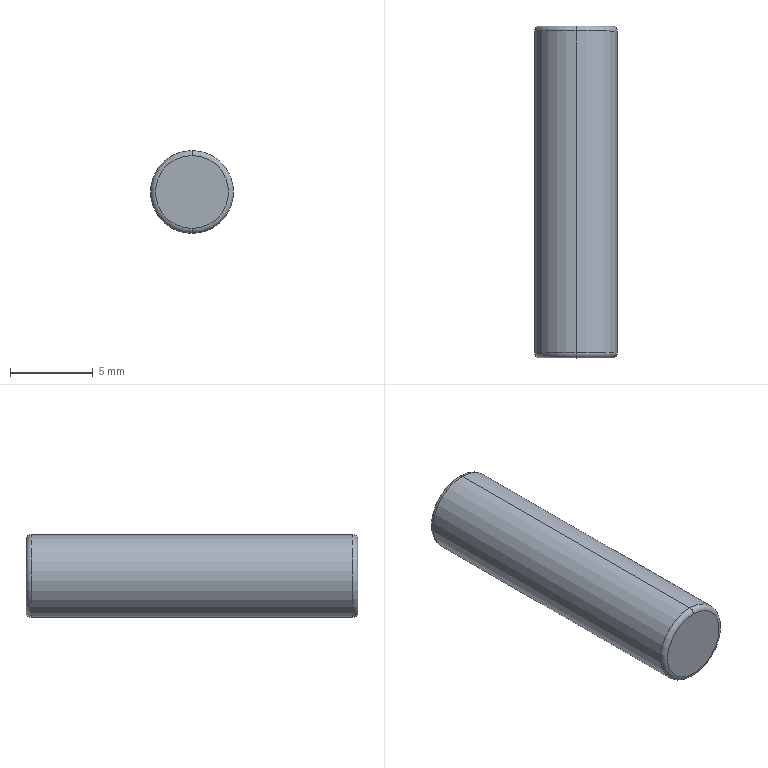Part | STEP file | 1 solid | 8 faces | box 5 x 20 x 5 mm | volume 392.109 mm3 | torus 4 | cylinder 2 | plane 2 | commonest cylinder face diameters 5 x2
STEP:
#1=CARTESIAN_POINT('',(0.,0.,0.));
#2=DIRECTION('',(0.,0.,1.));
#3=DIRECTION('',(1.,0.,0.));
#4=AXIS2_PLACEMENT_3D('',#1,#2,#3);
#5=CARTESIAN_POINT('',(0.,9.7,-2.5));
#6=VERTEX_POINT('',#5);
#7=CARTESIAN_POINT('',(0.,9.7,2.5));
#8=VERTEX_POINT('',#7);
#9=CARTESIAN_POINT('',(0.,9.7,0.));
#10=DIRECTION('',(0.,-1.,0.));
#11=DIRECTION('',(0.,0.,1.));
#12=AXIS2_PLACEMENT_3D('',#9,#10,#11);
#13=CIRCLE('',#12,2.5);
#14=CARTESIAN_POINT('',(0.,9.7,0.));
#15=DIRECTION('',(0.,1.,0.));
#16=DIRECTION('',(0.,0.,1.));
#17=AXIS2_PLACEMENT_3D('',#14,#15,#16);
#18=TOROIDAL_SURFACE('',#17,2.2,0.3);
#19=CARTESIAN_POINT('',(6.283,0.));
#20=DIRECTION('',(-1.,0.));
#21=VECTOR('',#20,1.);
#22=LINE('',#19,#21);
#23=(GEOMETRIC_REPRESENTATION_CONTEXT(2)PARAMETRIC_REPRESENTATION_CONTEXT()REPRESENTATION_CONTEXT('',''));
#24=DEFINITIONAL_REPRESENTATION('',(#22),#23);
#25=PCURVE('',#18,#24);
#26=CARTESIAN_POINT('',(0.,10.,0.));
#27=DIRECTION('',(0.,-1.,0.));
#28=DIRECTION('',(0.,0.,-1.));
#29=AXIS2_PLACEMENT_3D('',#26,#27,#28);
#30=CYLINDRICAL_SURFACE('',#29,2.5);
#31=CARTESIAN_POINT('',(-3.142,0.3));
#32=DIRECTION('',(1.,0.));
#33=VECTOR('',#32,1.);
#34=LINE('',#31,#33);
#35=(GEOMETRIC_REPRESENTATION_CONTEXT(2)PARAMETRIC_REPRESENTATION_CONTEXT()REPRESENTATION_CONTEXT('',''));
#36=DEFINITIONAL_REPRESENTATION('',(#34),#35);
#37=PCURVE('',#30,#36);
#38=SURFACE_CURVE('',#13,(#25,#37),.PCURVE_S1.);
#39=EDGE_CURVE('',#6,#8,#38,.T.);
#40=ORIENTED_EDGE('',*,*,#39,.F.);
#41=CARTESIAN_POINT('',(0.,10.,-2.2));
#42=VERTEX_POINT('',#41);
#43=CARTESIAN_POINT('',(0.,9.7,-2.2));
#44=DIRECTION('',(1.,0.,0.));
#45=DIRECTION('',(0.,0.,-1.));
#46=AXIS2_PLACEMENT_3D('',#43,#44,#45);
#47=CIRCLE('',#46,0.3);
#48=CARTESIAN_POINT('',(3.142,0.));
#49=DIRECTION('',(0.,1.));
#50=VECTOR('',#49,1.);
#51=LINE('',#48,#50);
#52=(GEOMETRIC_REPRESENTATION_CONTEXT(2)PARAMETRIC_REPRESENTATION_CONTEXT()REPRESENTATION_CONTEXT('',''));
#53=DEFINITIONAL_REPRESENTATION('',(#51),#52);
#54=PCURVE('',#18,#53);
#55=CARTESIAN_POINT('',(0.,9.7,0.));
#56=DIRECTION('',(0.,1.,0.));
#57=DIRECTION('',(0.,0.,1.));
#58=AXIS2_PLACEMENT_3D('',#55,#56,#57);
#59=TOROIDAL_SURFACE('',#58,2.2,0.3);
#60=CARTESIAN_POINT('',(3.142,0.));
#61=DIRECTION('',(0.,1.));
#62=VECTOR('',#61,1.);
#63=LINE('',#60,#62);
#64=(GEOMETRIC_REPRESENTATION_CONTEXT(2)PARAMETRIC_REPRESENTATION_CONTEXT()REPRESENTATION_CONTEXT('',''));
#65=DEFINITIONAL_REPRESENTATION('',(#63),#64);
#66=PCURVE('',#59,#65);
#67=SURFACE_CURVE('',#47,(#54,#66),.PCURVE_S1.);
#68=EDGE_CURVE('',#6,#42,#67,.T.);
#69=ORIENTED_EDGE('',*,*,#68,.T.);
#70=CARTESIAN_POINT('',(0.,10.,2.2));
#71=VERTEX_POINT('',#70);
#72=CARTESIAN_POINT('',(0.,10.,0.));
#73=DIRECTION('',(0.,1.,0.));
#74=DIRECTION('',(0.,0.,1.));
#75=AXIS2_PLACEMENT_3D('',#72,#73,#74);
#76=CIRCLE('',#75,2.2);
#77=CARTESIAN_POINT('',(0.,1.571));
#78=DIRECTION('',(1.,0.));
#79=VECTOR('',#78,1.);
#80=LINE('',#77,#79);
#81=(GEOMETRIC_REPRESENTATION_CONTEXT(2)PARAMETRIC_REPRESENTATION_CONTEXT()REPRESENTATION_CONTEXT('',''));
#82=DEFINITIONAL_REPRESENTATION('',(#80),#81);
#83=PCURVE('',#18,#82);
#84=CARTESIAN_POINT('',(0.,10.,0.));
#85=DIRECTION('',(0.,1.,0.));
#86=DIRECTION('',(0.,0.,1.));
#87=AXIS2_PLACEMENT_3D('',#84,#85,#86);
#88=PLANE('',#87);
#89=CARTESIAN_POINT('',(0.,0.));
#90=DIRECTION('',(1.,0.));
#91=AXIS2_PLACEMENT_2D('',#89,#90);
#92=CIRCLE('',#91,2.2);
#93=(GEOMETRIC_REPRESENTATION_CONTEXT(2)PARAMETRIC_REPRESENTATION_CONTEXT()REPRESENTATION_CONTEXT('',''));
#94=DEFINITIONAL_REPRESENTATION('',(#92),#93);
#95=PCURVE('',#88,#94);
#96=SURFACE_CURVE('',#76,(#83,#95),.PCURVE_S1.);
#97=EDGE_CURVE('',#71,#42,#96,.T.);
#98=ORIENTED_EDGE('',*,*,#97,.F.);
#99=CARTESIAN_POINT('',(0.,9.7,2.2));
#100=DIRECTION('',(-1.,0.,0.));
#101=DIRECTION('',(0.,0.,1.));
#102=AXIS2_PLACEMENT_3D('',#99,#100,#101);
#103=CIRCLE('',#102,0.3);
#104=CARTESIAN_POINT('',(0.,0.));
#105=DIRECTION('',(0.,1.));
#106=VECTOR('',#105,1.);
#107=LINE('',#104,#106);
#108=(GEOMETRIC_REPRESENTATION_CONTEXT(2)PARAMETRIC_REPRESENTATION_CONTEXT()REPRESENTATION_CONTEXT('',''));
#109=DEFINITIONAL_REPRESENTATION('',(#107),#108);
#110=PCURVE('',#18,#109);
#111=CARTESIAN_POINT('',(6.283,0.));
#112=DIRECTION('',(0.,1.));
#113=VECTOR('',#112,1.);
#114=LINE('',#111,#113);
#115=(GEOMETRIC_REPRESENTATION_CONTEXT(2)PARAMETRIC_REPRESENTATION_CONTEXT()REPRESENTATION_CONTEXT('',''));
#116=DEFINITIONAL_REPRESENTATION('',(#114),#115);
#117=PCURVE('',#59,#116);
#118=SURFACE_CURVE('',#103,(#110,#117),.PCURVE_S1.);
#119=EDGE_CURVE('',#8,#71,#118,.T.);
#120=ORIENTED_EDGE('',*,*,#119,.F.);
#121=EDGE_LOOP('',(#40,#69,#98,#120));
#122=FACE_BOUND('',#121,.T.);
#123=ADVANCED_FACE('',(#122),#18,.T.);
#124=CARTESIAN_POINT('',(0.,-10.,-2.2));
#125=VERTEX_POINT('',#124);
#126=CARTESIAN_POINT('',(0.,-10.,2.2));
#127=VERTEX_POINT('',#126);
#128=CARTESIAN_POINT('',(0.,-10.,0.));
#129=DIRECTION('',(0.,-1.,0.));
#130=DIRECTION('',(0.,0.,1.));
#131=AXIS2_PLACEMENT_3D('',#128,#129,#130);
#132=CIRCLE('',#131,2.2);
#133=CARTESIAN_POINT('',(0.,-9.7,0.));
#134=DIRECTION('',(0.,1.,0.));
#135=DIRECTION('',(0.,0.,1.));
#136=AXIS2_PLACEMENT_3D('',#133,#134,#135);
#137=TOROIDAL_SURFACE('',#136,2.2,0.3);
#138=CARTESIAN_POINT('',(6.283,4.712));
#139=DIRECTION('',(-1.,0.));
#140=VECTOR('',#139,1.);
#141=LINE('',#138,#140);
#142=(GEOMETRIC_REPRESENTATION_CONTEXT(2)PARAMETRIC_REPRESENTATION_CONTEXT()REPRESENTATION_CONTEXT('',''));
#143=DEFINITIONAL_REPRESENTATION('',(#141),#142);
#144=PCURVE('',#137,#143);
#145=CARTESIAN_POINT('',(0.,-10.,0.));
#146=DIRECTION('',(0.,1.,0.));
#147=DIRECTION('',(0.,0.,1.));
#148=AXIS2_PLACEMENT_3D('',#145,#146,#147);
#149=PLANE('',#148);
#150=CARTESIAN_POINT('',(2.2,0.));
#151=CARTESIAN_POINT('',(2.2,-3.811));
#152=CARTESIAN_POINT('',(-1.1,-1.905));
#153=CARTESIAN_POINT('',(-4.4,0.));
#154=CARTESIAN_POINT('',(-1.1,1.905));
#155=CARTESIAN_POINT('',(2.2,3.811));
#156=CARTESIAN_POINT('',(2.2,0.));
#157=(BOUNDED_CURVE()B_SPLINE_CURVE(2,(#150,#151,#152,#153,#154,#155,#156),.UNSPECIFIED.,.T.,.F.)B_SPLINE_CURVE_WITH_KNOTS((1,2,2,2,2,1),(-2.094,0.,2.094,4.189,6.283,8.378),.UNSPECIFIED.)CURVE()GEOMETRIC_REPRESENTATION_ITEM()RATIONAL_B_SPLINE_CURVE((1.,0.5,1.,0.5,1.,0.5,1.))REPRESENTATION_ITEM(''));
#158=(GEOMETRIC_REPRESENTATION_CONTEXT(2)PARAMETRIC_REPRESENTATION_CONTEXT()REPRESENTATION_CONTEXT('',''));
#159=DEFINITIONAL_REPRESENTATION('',(#157),#158);
#160=PCURVE('',#149,#159);
#161=SURFACE_CURVE('',#132,(#144,#160),.PCURVE_S1.);
#162=EDGE_CURVE('',#125,#127,#161,.T.);
#163=ORIENTED_EDGE('',*,*,#162,.F.);
#164=CARTESIAN_POINT('',(0.,-9.7,-2.5));
#165=VERTEX_POINT('',#164);
#166=CARTESIAN_POINT('',(0.,-9.7,-2.2));
#167=DIRECTION('',(1.,0.,0.));
#168=DIRECTION('',(0.,0.,-1.));
#169=AXIS2_PLACEMENT_3D('',#166,#167,#168);
#170=CIRCLE('',#169,0.3);
#171=CARTESIAN_POINT('',(3.142,0.));
#172=DIRECTION('',(0.,1.));
#173=VECTOR('',#172,1.);
#174=LINE('',#171,#173);
#175=(GEOMETRIC_REPRESENTATION_CONTEXT(2)PARAMETRIC_REPRESENTATION_CONTEXT()REPRESENTATION_CONTEXT('',''));
#176=DEFINITIONAL_REPRESENTATION('',(#174),#175);
#177=PCURVE('',#137,#176);
#178=CARTESIAN_POINT('',(0.,-9.7,0.));
#179=DIRECTION('',(0.,1.,0.));
#180=DIRECTION('',(0.,0.,1.));
#181=AXIS2_PLACEMENT_3D('',#178,#179,#180);
#182=TOROIDAL_SURFACE('',#181,2.2,0.3);
#183=CARTESIAN_POINT('',(3.142,0.));
#184=DIRECTION('',(0.,1.));
#185=VECTOR('',#184,1.);
#186=LINE('',#183,#185);
#187=(GEOMETRIC_REPRESENTATION_CONTEXT(2)PARAMETRIC_REPRESENTATION_CONTEXT()REPRESENTATION_CONTEXT('',''));
#188=DEFINITIONAL_REPRESENTATION('',(#186),#187);
#189=PCURVE('',#182,#188);
#190=SURFACE_CURVE('',#170,(#177,#189),.PCURVE_S1.);
#191=EDGE_CURVE('',#125,#165,#190,.T.);
#192=ORIENTED_EDGE('',*,*,#191,.T.);
#193=CARTESIAN_POINT('',(0.,-9.7,2.5));
#194=VERTEX_POINT('',#193);
#195=CARTESIAN_POINT('',(0.,-9.7,0.));
#196=DIRECTION('',(0.,1.,0.));
#197=DIRECTION('',(0.,0.,1.));
#198=AXIS2_PLACEMENT_3D('',#195,#196,#197);
#199=CIRCLE('',#198,2.5);
#200=CARTESIAN_POINT('',(0.,6.283));
#201=DIRECTION('',(1.,0.));
#202=VECTOR('',#201,1.);
#203=LINE('',#200,#202);
#204=(GEOMETRIC_REPRESENTATION_CONTEXT(2)PARAMETRIC_REPRESENTATION_CONTEXT()REPRESENTATION_CONTEXT('',''));
#205=DEFINITIONAL_REPRESENTATION('',(#203),#204);
#206=PCURVE('',#137,#205);
#207=CARTESIAN_POINT('',(3.142,19.7));
#208=DIRECTION('',(-1.,0.));
#209=VECTOR('',#208,1.);
#210=LINE('',#207,#209);
#211=(GEOMETRIC_REPRESENTATION_CONTEXT(2)PARAMETRIC_REPRESENTATION_CONTEXT()REPRESENTATION_CONTEXT('',''));
#212=DEFINITIONAL_REPRESENTATION('',(#210),#211);
#213=PCURVE('',#30,#212);
#214=SURFACE_CURVE('',#199,(#206,#213),.PCURVE_S1.);
#215=EDGE_CURVE('',#194,#165,#214,.T.);
#216=ORIENTED_EDGE('',*,*,#215,.F.);
#217=CARTESIAN_POINT('',(0.,-9.7,2.2));
#218=DIRECTION('',(-1.,0.,0.));
#219=DIRECTION('',(0.,0.,1.));
#220=AXIS2_PLACEMENT_3D('',#217,#218,#219);
#221=CIRCLE('',#220,0.3);
#222=CARTESIAN_POINT('',(0.,0.));
#223=DIRECTION('',(0.,1.));
#224=VECTOR('',#223,1.);
#225=LINE('',#222,#224);
#226=(GEOMETRIC_REPRESENTATION_CONTEXT(2)PARAMETRIC_REPRESENTATION_CONTEXT()REPRESENTATION_CONTEXT('',''));
#227=DEFINITIONAL_REPRESENTATION('',(#225),#226);
#228=PCURVE('',#137,#227);
#229=CARTESIAN_POINT('',(6.283,0.));
#230=DIRECTION('',(0.,1.));
#231=VECTOR('',#230,1.);
#232=LINE('',#229,#231);
#233=(GEOMETRIC_REPRESENTATION_CONTEXT(2)PARAMETRIC_REPRESENTATION_CONTEXT()REPRESENTATION_CONTEXT('',''));
#234=DEFINITIONAL_REPRESENTATION('',(#232),#233);
#235=PCURVE('',#182,#234);
#236=SURFACE_CURVE('',#221,(#228,#235),.PCURVE_S1.);
#237=EDGE_CURVE('',#127,#194,#236,.T.);
#238=ORIENTED_EDGE('',*,*,#237,.F.);
#239=EDGE_LOOP('',(#163,#192,#216,#238));
#240=FACE_BOUND('',#239,.T.);
#241=ADVANCED_FACE('',(#240),#137,.T.);
#242=ORIENTED_EDGE('',*,*,#39,.T.);
#243=CARTESIAN_POINT('',(0.,10.,2.5));
#244=DIRECTION('',(0.,-1.,0.));
#245=VECTOR('',#244,1.);
#246=LINE('',#243,#245);
#247=CARTESIAN_POINT('',(3.142,0.));
#248=DIRECTION('',(0.,1.));
#249=VECTOR('',#248,1.);
#250=LINE('',#247,#249);
#251=(GEOMETRIC_REPRESENTATION_CONTEXT(2)PARAMETRIC_REPRESENTATION_CONTEXT()REPRESENTATION_CONTEXT('',''));
#252=DEFINITIONAL_REPRESENTATION('',(#250),#251);
#253=PCURVE('',#30,#252);
#254=CARTESIAN_POINT('',(0.,10.,0.));
#255=DIRECTION('',(0.,-1.,0.));
#256=DIRECTION('',(0.,0.,-1.));
#257=AXIS2_PLACEMENT_3D('',#254,#255,#256);
#258=CYLINDRICAL_SURFACE('',#257,2.5);
#259=CARTESIAN_POINT('',(3.142,0.));
#260=DIRECTION('',(0.,1.));
#261=VECTOR('',#260,1.);
#262=LINE('',#259,#261);
#263=(GEOMETRIC_REPRESENTATION_CONTEXT(2)PARAMETRIC_REPRESENTATION_CONTEXT()REPRESENTATION_CONTEXT('',''));
#264=DEFINITIONAL_REPRESENTATION('',(#262),#263);
#265=PCURVE('',#258,#264);
#266=SURFACE_CURVE('',#246,(#253,#265),.PCURVE_S1.);
#267=EDGE_CURVE('',#8,#194,#266,.T.);
#268=ORIENTED_EDGE('',*,*,#267,.T.);
#269=ORIENTED_EDGE('',*,*,#215,.T.);
#270=CARTESIAN_POINT('',(0.,10.,-2.5));
#271=DIRECTION('',(0.,-1.,0.));
#272=VECTOR('',#271,1.);
#273=LINE('',#270,#272);
#274=CARTESIAN_POINT('',(0.,0.));
#275=DIRECTION('',(0.,1.));
#276=VECTOR('',#275,1.);
#277=LINE('',#274,#276);
#278=(GEOMETRIC_REPRESENTATION_CONTEXT(2)PARAMETRIC_REPRESENTATION_CONTEXT()REPRESENTATION_CONTEXT('',''));
#279=DEFINITIONAL_REPRESENTATION('',(#277),#278);
#280=PCURVE('',#30,#279);
#281=CARTESIAN_POINT('',(6.283,0.));
#282=DIRECTION('',(0.,1.));
#283=VECTOR('',#282,1.);
#284=LINE('',#281,#283);
#285=(GEOMETRIC_REPRESENTATION_CONTEXT(2)PARAMETRIC_REPRESENTATION_CONTEXT()REPRESENTATION_CONTEXT('',''));
#286=DEFINITIONAL_REPRESENTATION('',(#284),#285);
#287=PCURVE('',#258,#286);
#288=SURFACE_CURVE('',#273,(#280,#287),.PCURVE_S1.);
#289=EDGE_CURVE('',#6,#165,#288,.T.);
#290=ORIENTED_EDGE('',*,*,#289,.F.);
#291=EDGE_LOOP('',(#242,#268,#269,#290));
#292=FACE_BOUND('',#291,.T.);
#293=ADVANCED_FACE('',(#292),#30,.T.);
#294=ORIENTED_EDGE('',*,*,#267,.F.);
#295=CARTESIAN_POINT('',(0.,9.7,0.));
#296=DIRECTION('',(0.,-1.,0.));
#297=DIRECTION('',(0.,0.,1.));
#298=AXIS2_PLACEMENT_3D('',#295,#296,#297);
#299=CIRCLE('',#298,2.5);
#300=CARTESIAN_POINT('',(3.142,0.3));
#301=DIRECTION('',(1.,0.));
#302=VECTOR('',#301,1.);
#303=LINE('',#300,#302);
#304=(GEOMETRIC_REPRESENTATION_CONTEXT(2)PARAMETRIC_REPRESENTATION_CONTEXT()REPRESENTATION_CONTEXT('',''));
#305=DEFINITIONAL_REPRESENTATION('',(#303),#304);
#306=PCURVE('',#258,#305);
#307=CARTESIAN_POINT('',(6.283,0.));
#308=DIRECTION('',(-1.,0.));
#309=VECTOR('',#308,1.);
#310=LINE('',#307,#309);
#311=(GEOMETRIC_REPRESENTATION_CONTEXT(2)PARAMETRIC_REPRESENTATION_CONTEXT()REPRESENTATION_CONTEXT('',''));
#312=DEFINITIONAL_REPRESENTATION('',(#310),#311);
#313=PCURVE('',#59,#312);
#314=SURFACE_CURVE('',#299,(#306,#313),.PCURVE_S1.);
#315=EDGE_CURVE('',#8,#6,#314,.T.);
#316=ORIENTED_EDGE('',*,*,#315,.T.);
#317=ORIENTED_EDGE('',*,*,#289,.T.);
#318=CARTESIAN_POINT('',(0.,-9.7,0.));
#319=DIRECTION('',(0.,1.,0.));
#320=DIRECTION('',(0.,0.,1.));
#321=AXIS2_PLACEMENT_3D('',#318,#319,#320);
#322=CIRCLE('',#321,2.5);
#323=CARTESIAN_POINT('',(9.425,19.7));
#324=DIRECTION('',(-1.,0.));
#325=VECTOR('',#324,1.);
#326=LINE('',#323,#325);
#327=(GEOMETRIC_REPRESENTATION_CONTEXT(2)PARAMETRIC_REPRESENTATION_CONTEXT()REPRESENTATION_CONTEXT('',''));
#328=DEFINITIONAL_REPRESENTATION('',(#326),#327);
#329=PCURVE('',#258,#328);
#330=CARTESIAN_POINT('',(0.,6.283));
#331=DIRECTION('',(1.,0.));
#332=VECTOR('',#331,1.);
#333=LINE('',#330,#332);
#334=(GEOMETRIC_REPRESENTATION_CONTEXT(2)PARAMETRIC_REPRESENTATION_CONTEXT()REPRESENTATION_CONTEXT('',''));
#335=DEFINITIONAL_REPRESENTATION('',(#333),#334);
#336=PCURVE('',#182,#335);
#337=SURFACE_CURVE('',#322,(#329,#336),.PCURVE_S1.);
#338=EDGE_CURVE('',#165,#194,#337,.T.);
#339=ORIENTED_EDGE('',*,*,#338,.T.);
#340=EDGE_LOOP('',(#294,#316,#317,#339));
#341=FACE_BOUND('',#340,.T.);
#342=ADVANCED_FACE('',(#341),#258,.T.);
#343=ORIENTED_EDGE('',*,*,#97,.T.);
#344=CARTESIAN_POINT('',(0.,10.,0.));
#345=DIRECTION('',(0.,1.,0.));
#346=DIRECTION('',(0.,0.,1.));
#347=AXIS2_PLACEMENT_3D('',#344,#345,#346);
#348=CIRCLE('',#347,2.2);
#349=CARTESIAN_POINT('',(0.,0.));
#350=DIRECTION('',(1.,0.));
#351=AXIS2_PLACEMENT_2D('',#349,#350);
#352=CIRCLE('',#351,2.2);
#353=(GEOMETRIC_REPRESENTATION_CONTEXT(2)PARAMETRIC_REPRESENTATION_CONTEXT()REPRESENTATION_CONTEXT('',''));
#354=DEFINITIONAL_REPRESENTATION('',(#352),#353);
#355=PCURVE('',#88,#354);
#356=CARTESIAN_POINT('',(0.,1.571));
#357=DIRECTION('',(1.,0.));
#358=VECTOR('',#357,1.);
#359=LINE('',#356,#358);
#360=(GEOMETRIC_REPRESENTATION_CONTEXT(2)PARAMETRIC_REPRESENTATION_CONTEXT()REPRESENTATION_CONTEXT('',''));
#361=DEFINITIONAL_REPRESENTATION('',(#359),#360);
#362=PCURVE('',#59,#361);
#363=SURFACE_CURVE('',#348,(#355,#362),.PCURVE_S1.);
#364=EDGE_CURVE('',#42,#71,#363,.T.);
#365=ORIENTED_EDGE('',*,*,#364,.T.);
#366=EDGE_LOOP('',(#343,#365));
#367=FACE_BOUND('',#366,.T.);
#368=ADVANCED_FACE('',(#367),#88,.T.);
#369=CARTESIAN_POINT('',(0.,-10.,0.));
#370=DIRECTION('',(0.,-1.,0.));
#371=DIRECTION('',(0.,0.,1.));
#372=AXIS2_PLACEMENT_3D('',#369,#370,#371);
#373=CIRCLE('',#372,2.2);
#374=CARTESIAN_POINT('',(2.2,0.));
#375=CARTESIAN_POINT('',(2.2,-3.811));
#376=CARTESIAN_POINT('',(-1.1,-1.905));
#377=CARTESIAN_POINT('',(-4.4,0.));
#378=CARTESIAN_POINT('',(-1.1,1.905));
#379=CARTESIAN_POINT('',(2.2,3.811));
#380=CARTESIAN_POINT('',(2.2,0.));
#381=(BOUNDED_CURVE()B_SPLINE_CURVE(2,(#374,#375,#376,#377,#378,#379,#380),.UNSPECIFIED.,.T.,.F.)B_SPLINE_CURVE_WITH_KNOTS((1,2,2,2,2,1),(-2.094,0.,2.094,4.189,6.283,8.378),.UNSPECIFIED.)CURVE()GEOMETRIC_REPRESENTATION_ITEM()RATIONAL_B_SPLINE_CURVE((1.,0.5,1.,0.5,1.,0.5,1.))REPRESENTATION_ITEM(''));
#382=(GEOMETRIC_REPRESENTATION_CONTEXT(2)PARAMETRIC_REPRESENTATION_CONTEXT()REPRESENTATION_CONTEXT('',''));
#383=DEFINITIONAL_REPRESENTATION('',(#381),#382);
#384=PCURVE('',#149,#383);
#385=CARTESIAN_POINT('',(6.283,4.712));
#386=DIRECTION('',(-1.,0.));
#387=VECTOR('',#386,1.);
#388=LINE('',#385,#387);
#389=(GEOMETRIC_REPRESENTATION_CONTEXT(2)PARAMETRIC_REPRESENTATION_CONTEXT()REPRESENTATION_CONTEXT('',''));
#390=DEFINITIONAL_REPRESENTATION('',(#388),#389);
#391=PCURVE('',#182,#390);
#392=SURFACE_CURVE('',#373,(#384,#391),.PCURVE_S1.);
#393=EDGE_CURVE('',#127,#125,#392,.T.);
#394=ORIENTED_EDGE('',*,*,#393,.T.);
#395=ORIENTED_EDGE('',*,*,#162,.T.);
#396=EDGE_LOOP('',(#394,#395));
#397=FACE_BOUND('',#396,.T.);
#398=ADVANCED_FACE('',(#397),#149,.F.);
#399=ORIENTED_EDGE('',*,*,#191,.F.);
#400=ORIENTED_EDGE('',*,*,#393,.F.);
#401=ORIENTED_EDGE('',*,*,#237,.T.);
#402=ORIENTED_EDGE('',*,*,#338,.F.);
#403=EDGE_LOOP('',(#399,#400,#401,#402));
#404=FACE_BOUND('',#403,.T.);
#405=ADVANCED_FACE('',(#404),#182,.T.);
#406=ORIENTED_EDGE('',*,*,#68,.F.);
#407=ORIENTED_EDGE('',*,*,#315,.F.);
#408=ORIENTED_EDGE('',*,*,#119,.T.);
#409=ORIENTED_EDGE('',*,*,#364,.F.);
#410=EDGE_LOOP('',(#406,#407,#408,#409));
#411=FACE_BOUND('',#410,.T.);
#412=ADVANCED_FACE('',(#411),#59,.T.);
#413=CLOSED_SHELL('',(#123,#241,#293,#342,#368,#398,#405,#412));
#414=MANIFOLD_SOLID_BREP('',#413);
#415=(LENGTH_UNIT()NAMED_UNIT(*)SI_UNIT(.MILLI.,.METRE.));
#416=UNCERTAINTY_MEASURE_WITH_UNIT(LENGTH_MEASURE(0.0000001),#415,'','');
#417=(NAMED_UNIT(*)PLANE_ANGLE_UNIT()SI_UNIT($,.RADIAN.));
#418=(NAMED_UNIT(*)SI_UNIT($,.STERADIAN.)SOLID_ANGLE_UNIT());
#419=(GEOMETRIC_REPRESENTATION_CONTEXT(3)GLOBAL_UNCERTAINTY_ASSIGNED_CONTEXT((#416))GLOBAL_UNIT_ASSIGNED_CONTEXT((#415,#417,#418))REPRESENTATION_CONTEXT('',''));
#420=ADVANCED_BREP_SHAPE_REPRESENTATION('',(#4,#414),#419);